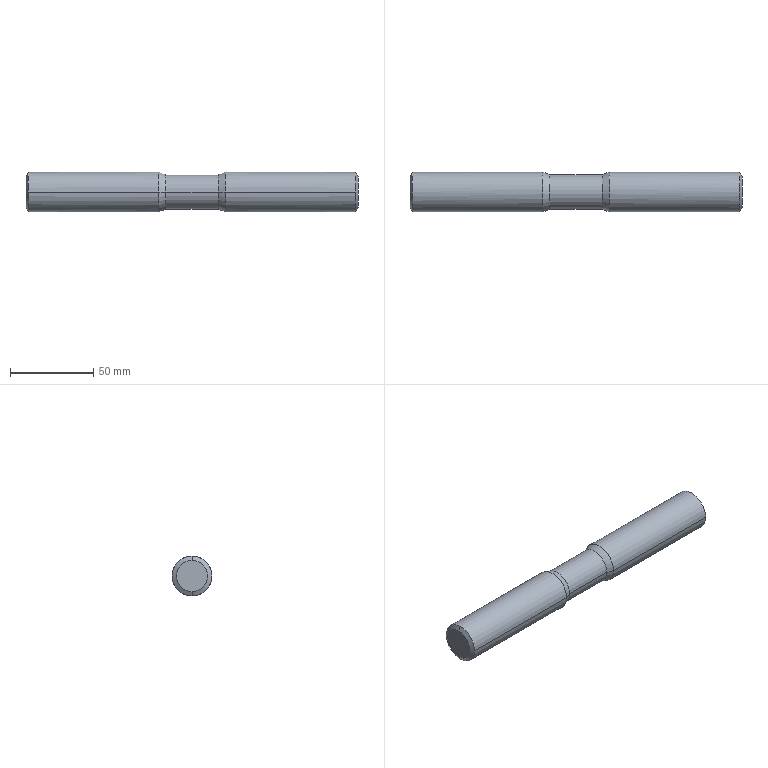Part | STEP file | GB/T901-1988 double-end stud, grade B, M24×200 | 1 solid | 16 faces | box 200 x 24 x 24 mm | volume 86144 mm3 | cone 8 | cylinder 6 | plane 2 | commonest cylinder face diameters 24 x4 20.784 x2
STEP:
#1=CARTESIAN_POINT('',(0.,0.,0.));
#2=DIRECTION('',(0.,0.,1.));
#3=DIRECTION('',(1.,0.,0.));
#4=AXIS2_PLACEMENT_3D('',#1,#2,#3);
#5=CARTESIAN_POINT('',(100.,0.,-9.402));
#6=VERTEX_POINT('',#5);
#7=CARTESIAN_POINT('',(100.,0.,9.402));
#8=VERTEX_POINT('',#7);
#9=CARTESIAN_POINT('',(100.,0.,0.));
#10=DIRECTION('',(-1.,0.,0.));
#11=DIRECTION('',(0.,0.,1.));
#12=AXIS2_PLACEMENT_3D('',#9,#10,#11);
#13=CIRCLE('',#12,9.402);
#14=CARTESIAN_POINT('',(100.,0.,0.));
#15=DIRECTION('',(-1.,0.,0.));
#16=DIRECTION('',(0.,0.,-1.));
#17=AXIS2_PLACEMENT_3D('',#14,#15,#16);
#18=CONICAL_SURFACE('',#17,9.402,1.047);
#19=CARTESIAN_POINT('',(-3.142,0.));
#20=DIRECTION('',(1.,0.));
#21=VECTOR('',#20,1.);
#22=LINE('',#19,#21);
#23=(GEOMETRIC_REPRESENTATION_CONTEXT(2)PARAMETRIC_REPRESENTATION_CONTEXT()REPRESENTATION_CONTEXT('',''));
#24=DEFINITIONAL_REPRESENTATION('',(#22),#23);
#25=PCURVE('',#18,#24);
#26=CARTESIAN_POINT('',(100.,12.,0.));
#27=DIRECTION('',(-1.,0.,0.));
#28=DIRECTION('',(0.,1.,0.));
#29=AXIS2_PLACEMENT_3D('',#26,#27,#28);
#30=PLANE('',#29);
#31=CARTESIAN_POINT('',(-12.,0.));
#32=DIRECTION('',(0.,-1.));
#33=AXIS2_PLACEMENT_2D('',#31,#32);
#34=CIRCLE('',#33,9.402);
#35=(GEOMETRIC_REPRESENTATION_CONTEXT(2)PARAMETRIC_REPRESENTATION_CONTEXT()REPRESENTATION_CONTEXT('',''));
#36=DEFINITIONAL_REPRESENTATION('',(#34),#35);
#37=PCURVE('',#30,#36);
#38=SURFACE_CURVE('',#13,(#25,#37),.PCURVE_S1.);
#39=EDGE_CURVE('',#6,#8,#38,.T.);
#40=ORIENTED_EDGE('',*,*,#39,.T.);
#41=CARTESIAN_POINT('',(98.5,0.,12.));
#42=VERTEX_POINT('',#41);
#43=CARTESIAN_POINT('',(100.,0.,9.402));
#44=DIRECTION('',(-0.5,0.,0.866));
#45=VECTOR('',#44,1.);
#46=LINE('',#43,#45);
#47=CARTESIAN_POINT('',(3.142,0.));
#48=DIRECTION('',(0.,1.));
#49=VECTOR('',#48,1.);
#50=LINE('',#47,#49);
#51=(GEOMETRIC_REPRESENTATION_CONTEXT(2)PARAMETRIC_REPRESENTATION_CONTEXT()REPRESENTATION_CONTEXT('',''));
#52=DEFINITIONAL_REPRESENTATION('',(#50),#51);
#53=PCURVE('',#18,#52);
#54=CARTESIAN_POINT('',(100.,0.,0.));
#55=DIRECTION('',(-1.,0.,0.));
#56=DIRECTION('',(0.,0.,-1.));
#57=AXIS2_PLACEMENT_3D('',#54,#55,#56);
#58=CONICAL_SURFACE('',#57,9.402,1.047);
#59=CARTESIAN_POINT('',(3.142,0.));
#60=DIRECTION('',(0.,1.));
#61=VECTOR('',#60,1.);
#62=LINE('',#59,#61);
#63=(GEOMETRIC_REPRESENTATION_CONTEXT(2)PARAMETRIC_REPRESENTATION_CONTEXT()REPRESENTATION_CONTEXT('',''));
#64=DEFINITIONAL_REPRESENTATION('',(#62),#63);
#65=PCURVE('',#58,#64);
#66=SURFACE_CURVE('',#46,(#53,#65),.PCURVE_S1.);
#67=EDGE_CURVE('',#8,#42,#66,.T.);
#68=ORIENTED_EDGE('',*,*,#67,.T.);
#69=CARTESIAN_POINT('',(98.5,-12.,0.));
#70=VERTEX_POINT('',#69);
#71=CARTESIAN_POINT('',(98.5,0.,0.));
#72=DIRECTION('',(-1.,0.,0.));
#73=DIRECTION('',(0.,0.,1.));
#74=AXIS2_PLACEMENT_3D('',#71,#72,#73);
#75=CIRCLE('',#74,12.);
#76=CARTESIAN_POINT('',(-3.142,1.5));
#77=DIRECTION('',(1.,0.));
#78=VECTOR('',#77,1.);
#79=LINE('',#76,#78);
#80=(GEOMETRIC_REPRESENTATION_CONTEXT(2)PARAMETRIC_REPRESENTATION_CONTEXT()REPRESENTATION_CONTEXT('',''));
#81=DEFINITIONAL_REPRESENTATION('',(#79),#80);
#82=PCURVE('',#18,#81);
#83=CARTESIAN_POINT('',(100.,0.,0.));
#84=DIRECTION('',(1.,0.,0.));
#85=DIRECTION('',(0.,-1.,0.));
#86=AXIS2_PLACEMENT_3D('',#83,#84,#85);
#87=CYLINDRICAL_SURFACE('',#86,12.);
#88=CARTESIAN_POINT('',(10.996,-1.5));
#89=DIRECTION('',(-1.,0.));
#90=VECTOR('',#89,1.);
#91=LINE('',#88,#90);
#92=(GEOMETRIC_REPRESENTATION_CONTEXT(2)PARAMETRIC_REPRESENTATION_CONTEXT()REPRESENTATION_CONTEXT('',''));
#93=DEFINITIONAL_REPRESENTATION('',(#91),#92);
#94=PCURVE('',#87,#93);
#95=SURFACE_CURVE('',#75,(#82,#94),.PCURVE_S1.);
#96=EDGE_CURVE('',#70,#42,#95,.T.);
#97=ORIENTED_EDGE('',*,*,#96,.F.);
#98=CARTESIAN_POINT('',(98.5,0.,-12.));
#99=VERTEX_POINT('',#98);
#100=CARTESIAN_POINT('',(98.5,0.,0.));
#101=DIRECTION('',(-1.,0.,0.));
#102=DIRECTION('',(0.,0.,1.));
#103=AXIS2_PLACEMENT_3D('',#100,#101,#102);
#104=CIRCLE('',#103,12.);
#105=CARTESIAN_POINT('',(-3.142,1.5));
#106=DIRECTION('',(1.,0.));
#107=VECTOR('',#106,1.);
#108=LINE('',#105,#107);
#109=(GEOMETRIC_REPRESENTATION_CONTEXT(2)PARAMETRIC_REPRESENTATION_CONTEXT()REPRESENTATION_CONTEXT('',''));
#110=DEFINITIONAL_REPRESENTATION('',(#108),#109);
#111=PCURVE('',#18,#110);
#112=CARTESIAN_POINT('',(100.,0.,0.));
#113=DIRECTION('',(1.,0.,0.));
#114=DIRECTION('',(0.,-1.,0.));
#115=AXIS2_PLACEMENT_3D('',#112,#113,#114);
#116=CYLINDRICAL_SURFACE('',#115,12.);
#117=CARTESIAN_POINT('',(4.712,-1.5));
#118=DIRECTION('',(-1.,0.));
#119=VECTOR('',#118,1.);
#120=LINE('',#117,#119);
#121=(GEOMETRIC_REPRESENTATION_CONTEXT(2)PARAMETRIC_REPRESENTATION_CONTEXT()REPRESENTATION_CONTEXT('',''));
#122=DEFINITIONAL_REPRESENTATION('',(#120),#121);
#123=PCURVE('',#116,#122);
#124=SURFACE_CURVE('',#104,(#111,#123),.PCURVE_S1.);
#125=EDGE_CURVE('',#99,#70,#124,.T.);
#126=ORIENTED_EDGE('',*,*,#125,.F.);
#127=CARTESIAN_POINT('',(100.,0.,-9.402));
#128=DIRECTION('',(-0.5,0.,-0.866));
#129=VECTOR('',#128,1.);
#130=LINE('',#127,#129);
#131=CARTESIAN_POINT('',(0.,0.));
#132=DIRECTION('',(0.,1.));
#133=VECTOR('',#132,1.);
#134=LINE('',#131,#133);
#135=(GEOMETRIC_REPRESENTATION_CONTEXT(2)PARAMETRIC_REPRESENTATION_CONTEXT()REPRESENTATION_CONTEXT('',''));
#136=DEFINITIONAL_REPRESENTATION('',(#134),#135);
#137=PCURVE('',#18,#136);
#138=CARTESIAN_POINT('',(6.283,0.));
#139=DIRECTION('',(0.,1.));
#140=VECTOR('',#139,1.);
#141=LINE('',#138,#140);
#142=(GEOMETRIC_REPRESENTATION_CONTEXT(2)PARAMETRIC_REPRESENTATION_CONTEXT()REPRESENTATION_CONTEXT('',''));
#143=DEFINITIONAL_REPRESENTATION('',(#141),#142);
#144=PCURVE('',#58,#143);
#145=SURFACE_CURVE('',#130,(#137,#144),.PCURVE_S1.);
#146=EDGE_CURVE('',#6,#99,#145,.T.);
#147=ORIENTED_EDGE('',*,*,#146,.F.);
#148=EDGE_LOOP('',(#40,#68,#97,#126,#147));
#149=FACE_BOUND('',#148,.T.);
#150=ADVANCED_FACE('',(#149),#18,.T.);
#151=CARTESIAN_POINT('',(15.8,10.392,0.));
#152=VERTEX_POINT('',#151);
#153=CARTESIAN_POINT('',(15.8,-10.392,0.));
#154=VERTEX_POINT('',#153);
#155=CARTESIAN_POINT('',(15.8,0.,0.));
#156=DIRECTION('',(-1.,0.,0.));
#157=DIRECTION('',(0.,-1.,0.));
#158=AXIS2_PLACEMENT_3D('',#155,#156,#157);
#159=CIRCLE('',#158,10.392);
#160=CARTESIAN_POINT('',(15.8,0.,0.));
#161=DIRECTION('',(1.,0.,0.));
#162=DIRECTION('',(0.,-1.,0.));
#163=AXIS2_PLACEMENT_3D('',#160,#161,#162);
#164=CONICAL_SURFACE('',#163,10.392,0.3656);
#165=CARTESIAN_POINT('',(6.283,0.));
#166=DIRECTION('',(-1.,0.));
#167=VECTOR('',#166,1.);
#168=LINE('',#165,#167);
#169=(GEOMETRIC_REPRESENTATION_CONTEXT(2)PARAMETRIC_REPRESENTATION_CONTEXT()REPRESENTATION_CONTEXT('',''));
#170=DEFINITIONAL_REPRESENTATION('',(#168),#169);
#171=PCURVE('',#164,#170);
#172=CARTESIAN_POINT('',(-100.,0.,0.));
#173=DIRECTION('',(-1.,0.,0.));
#174=DIRECTION('',(0.,-1.,0.));
#175=AXIS2_PLACEMENT_3D('',#172,#173,#174);
#176=CYLINDRICAL_SURFACE('',#175,10.392);
#177=CARTESIAN_POINT('',(0.,-115.8));
#178=DIRECTION('',(1.,0.));
#179=VECTOR('',#178,1.);
#180=LINE('',#177,#179);
#181=(GEOMETRIC_REPRESENTATION_CONTEXT(2)PARAMETRIC_REPRESENTATION_CONTEXT()REPRESENTATION_CONTEXT('',''));
#182=DEFINITIONAL_REPRESENTATION('',(#180),#181);
#183=PCURVE('',#176,#182);
#184=SURFACE_CURVE('',#159,(#171,#183),.PCURVE_S1.);
#185=EDGE_CURVE('',#152,#154,#184,.T.);
#186=ORIENTED_EDGE('',*,*,#185,.F.);
#187=CARTESIAN_POINT('',(20.,12.,0.));
#188=VERTEX_POINT('',#187);
#189=CARTESIAN_POINT('',(15.8,10.392,0.));
#190=DIRECTION('',(0.9339,0.3575,0.));
#191=VECTOR('',#190,1.);
#192=LINE('',#189,#191);
#193=CARTESIAN_POINT('',(3.142,0.));
#194=DIRECTION('',(0.,1.));
#195=VECTOR('',#194,1.);
#196=LINE('',#193,#195);
#197=(GEOMETRIC_REPRESENTATION_CONTEXT(2)PARAMETRIC_REPRESENTATION_CONTEXT()REPRESENTATION_CONTEXT('',''));
#198=DEFINITIONAL_REPRESENTATION('',(#196),#197);
#199=PCURVE('',#164,#198);
#200=CARTESIAN_POINT('',(15.8,0.,0.));
#201=DIRECTION('',(1.,0.,0.));
#202=DIRECTION('',(0.,-1.,0.));
#203=AXIS2_PLACEMENT_3D('',#200,#201,#202);
#204=CONICAL_SURFACE('',#203,10.392,0.3656);
#205=CARTESIAN_POINT('',(3.142,0.));
#206=DIRECTION('',(0.,1.));
#207=VECTOR('',#206,1.);
#208=LINE('',#205,#207);
#209=(GEOMETRIC_REPRESENTATION_CONTEXT(2)PARAMETRIC_REPRESENTATION_CONTEXT()REPRESENTATION_CONTEXT('',''));
#210=DEFINITIONAL_REPRESENTATION('',(#208),#209);
#211=PCURVE('',#204,#210);
#212=SURFACE_CURVE('',#192,(#199,#211),.PCURVE_S1.);
#213=EDGE_CURVE('',#152,#188,#212,.T.);
#214=ORIENTED_EDGE('',*,*,#213,.T.);
#215=CARTESIAN_POINT('',(20.,-12.,0.));
#216=VERTEX_POINT('',#215);
#217=CARTESIAN_POINT('',(20.,0.,0.));
#218=DIRECTION('',(-1.,0.,0.));
#219=DIRECTION('',(0.,-1.,0.));
#220=AXIS2_PLACEMENT_3D('',#217,#218,#219);
#221=CIRCLE('',#220,12.);
#222=CARTESIAN_POINT('',(6.283,4.2));
#223=DIRECTION('',(-1.,0.));
#224=VECTOR('',#223,1.);
#225=LINE('',#222,#224);
#226=(GEOMETRIC_REPRESENTATION_CONTEXT(2)PARAMETRIC_REPRESENTATION_CONTEXT()REPRESENTATION_CONTEXT('',''));
#227=DEFINITIONAL_REPRESENTATION('',(#225),#226);
#228=PCURVE('',#164,#227);
#229=CARTESIAN_POINT('',(6.283,-80.));
#230=DIRECTION('',(-1.,0.));
#231=VECTOR('',#230,1.);
#232=LINE('',#229,#231);
#233=(GEOMETRIC_REPRESENTATION_CONTEXT(2)PARAMETRIC_REPRESENTATION_CONTEXT()REPRESENTATION_CONTEXT('',''));
#234=DEFINITIONAL_REPRESENTATION('',(#232),#233);
#235=PCURVE('',#116,#234);
#236=SURFACE_CURVE('',#221,(#228,#235),.PCURVE_S1.);
#237=EDGE_CURVE('',#188,#216,#236,.T.);
#238=ORIENTED_EDGE('',*,*,#237,.T.);
#239=CARTESIAN_POINT('',(15.8,-10.392,0.));
#240=DIRECTION('',(0.9339,-0.3575,0.));
#241=VECTOR('',#240,1.);
#242=LINE('',#239,#241);
#243=CARTESIAN_POINT('',(0.,0.));
#244=DIRECTION('',(0.,1.));
#245=VECTOR('',#244,1.);
#246=LINE('',#243,#245);
#247=(GEOMETRIC_REPRESENTATION_CONTEXT(2)PARAMETRIC_REPRESENTATION_CONTEXT()REPRESENTATION_CONTEXT('',''));
#248=DEFINITIONAL_REPRESENTATION('',(#246),#247);
#249=PCURVE('',#164,#248);
#250=CARTESIAN_POINT('',(6.283,0.));
#251=DIRECTION('',(0.,1.));
#252=VECTOR('',#251,1.);
#253=LINE('',#250,#252);
#254=(GEOMETRIC_REPRESENTATION_CONTEXT(2)PARAMETRIC_REPRESENTATION_CONTEXT()REPRESENTATION_CONTEXT('',''));
#255=DEFINITIONAL_REPRESENTATION('',(#253),#254);
#256=PCURVE('',#204,#255);
#257=SURFACE_CURVE('',#242,(#249,#256),.PCURVE_S1.);
#258=EDGE_CURVE('',#154,#216,#257,.T.);
#259=ORIENTED_EDGE('',*,*,#258,.F.);
#260=EDGE_LOOP('',(#186,#214,#238,#259));
#261=FACE_BOUND('',#260,.T.);
#262=ADVANCED_FACE('',(#261),#164,.T.);
#263=ORIENTED_EDGE('',*,*,#237,.F.);
#264=CARTESIAN_POINT('',(98.5,12.,0.));
#265=VERTEX_POINT('',#264);
#266=CARTESIAN_POINT('',(100.,12.,0.));
#267=DIRECTION('',(1.,0.,0.));
#268=VECTOR('',#267,1.);
#269=LINE('',#266,#268);
#270=CARTESIAN_POINT('',(3.142,0.));
#271=DIRECTION('',(0.,1.));
#272=VECTOR('',#271,1.);
#273=LINE('',#270,#272);
#274=(GEOMETRIC_REPRESENTATION_CONTEXT(2)PARAMETRIC_REPRESENTATION_CONTEXT()REPRESENTATION_CONTEXT('',''));
#275=DEFINITIONAL_REPRESENTATION('',(#273),#274);
#276=PCURVE('',#116,#275);
#277=CARTESIAN_POINT('',(3.142,0.));
#278=DIRECTION('',(0.,1.));
#279=VECTOR('',#278,1.);
#280=LINE('',#277,#279);
#281=(GEOMETRIC_REPRESENTATION_CONTEXT(2)PARAMETRIC_REPRESENTATION_CONTEXT()REPRESENTATION_CONTEXT('',''));
#282=DEFINITIONAL_REPRESENTATION('',(#280),#281);
#283=PCURVE('',#87,#282);
#284=SURFACE_CURVE('',#269,(#276,#283),.PCURVE_S1.);
#285=EDGE_CURVE('',#188,#265,#284,.T.);
#286=ORIENTED_EDGE('',*,*,#285,.T.);
#287=CARTESIAN_POINT('',(98.5,0.,0.));
#288=DIRECTION('',(-1.,0.,0.));
#289=DIRECTION('',(0.,0.,1.));
#290=AXIS2_PLACEMENT_3D('',#287,#288,#289);
#291=CIRCLE('',#290,12.);
#292=CARTESIAN_POINT('',(4.712,-1.5));
#293=DIRECTION('',(-1.,0.));
#294=VECTOR('',#293,1.);
#295=LINE('',#292,#294);
#296=(GEOMETRIC_REPRESENTATION_CONTEXT(2)PARAMETRIC_REPRESENTATION_CONTEXT()REPRESENTATION_CONTEXT('',''));
#297=DEFINITIONAL_REPRESENTATION('',(#295),#296);
#298=PCURVE('',#116,#297);
#299=CARTESIAN_POINT('',(3.142,1.5));
#300=DIRECTION('',(1.,0.));
#301=VECTOR('',#300,1.);
#302=LINE('',#299,#301);
#303=(GEOMETRIC_REPRESENTATION_CONTEXT(2)PARAMETRIC_REPRESENTATION_CONTEXT()REPRESENTATION_CONTEXT('',''));
#304=DEFINITIONAL_REPRESENTATION('',(#302),#303);
#305=PCURVE('',#58,#304);
#306=SURFACE_CURVE('',#291,(#298,#305),.PCURVE_S1.);
#307=EDGE_CURVE('',#265,#99,#306,.T.);
#308=ORIENTED_EDGE('',*,*,#307,.T.);
#309=ORIENTED_EDGE('',*,*,#125,.T.);
#310=CARTESIAN_POINT('',(100.,-12.,0.));
#311=DIRECTION('',(1.,0.,0.));
#312=VECTOR('',#311,1.);
#313=LINE('',#310,#312);
#314=CARTESIAN_POINT('',(0.,0.));
#315=DIRECTION('',(0.,1.));
#316=VECTOR('',#315,1.);
#317=LINE('',#314,#316);
#318=(GEOMETRIC_REPRESENTATION_CONTEXT(2)PARAMETRIC_REPRESENTATION_CONTEXT()REPRESENTATION_CONTEXT('',''));
#319=DEFINITIONAL_REPRESENTATION('',(#317),#318);
#320=PCURVE('',#116,#319);
#321=CARTESIAN_POINT('',(6.283,0.));
#322=DIRECTION('',(0.,1.));
#323=VECTOR('',#322,1.);
#324=LINE('',#321,#323);
#325=(GEOMETRIC_REPRESENTATION_CONTEXT(2)PARAMETRIC_REPRESENTATION_CONTEXT()REPRESENTATION_CONTEXT('',''));
#326=DEFINITIONAL_REPRESENTATION('',(#324),#325);
#327=PCURVE('',#87,#326);
#328=SURFACE_CURVE('',#313,(#320,#327),.PCURVE_S1.);
#329=EDGE_CURVE('',#216,#70,#328,.T.);
#330=ORIENTED_EDGE('',*,*,#329,.F.);
#331=EDGE_LOOP('',(#263,#286,#308,#309,#330));
#332=FACE_BOUND('',#331,.T.);
#333=ADVANCED_FACE('',(#332),#116,.T.);
#334=CARTESIAN_POINT('',(-100.,0.,9.402));
#335=VERTEX_POINT('',#334);
#336=CARTESIAN_POINT('',(-100.,0.,-9.402));
#337=VERTEX_POINT('',#336);
#338=CARTESIAN_POINT('',(-100.,0.,0.));
#339=DIRECTION('',(-1.,0.,0.));
#340=DIRECTION('',(0.,0.,1.));
#341=AXIS2_PLACEMENT_3D('',#338,#339,#340);
#342=CIRCLE('',#341,9.402);
#343=CARTESIAN_POINT('',(-100.,0.,0.));
#344=DIRECTION('',(1.,0.,0.));
#345=DIRECTION('',(0.,0.,-1.));
#346=AXIS2_PLACEMENT_3D('',#343,#344,#345);
#347=CONICAL_SURFACE('',#346,9.402,1.047);
#348=CARTESIAN_POINT('',(3.142,0.));
#349=DIRECTION('',(-1.,0.));
#350=VECTOR('',#349,1.);
#351=LINE('',#348,#350);
#352=(GEOMETRIC_REPRESENTATION_CONTEXT(2)PARAMETRIC_REPRESENTATION_CONTEXT()REPRESENTATION_CONTEXT('',''));
#353=DEFINITIONAL_REPRESENTATION('',(#351),#352);
#354=PCURVE('',#347,#353);
#355=CARTESIAN_POINT('',(-100.,12.,0.));
#356=DIRECTION('',(1.,0.,0.));
#357=DIRECTION('',(0.,1.,0.));
#358=AXIS2_PLACEMENT_3D('',#355,#356,#357);
#359=PLANE('',#358);
#360=CARTESIAN_POINT('',(-12.,9.402));
#361=CARTESIAN_POINT('',(4.285,9.402));
#362=CARTESIAN_POINT('',(-3.858,-4.701));
#363=CARTESIAN_POINT('',(-12.,-18.804));
#364=CARTESIAN_POINT('',(-20.142,-4.701));
#365=CARTESIAN_POINT('',(-28.285,9.402));
#366=CARTESIAN_POINT('',(-12.,9.402));
#367=(BOUNDED_CURVE()B_SPLINE_CURVE(2,(#360,#361,#362,#363,#364,#365,#366),.UNSPECIFIED.,.T.,.F.)B_SPLINE_CURVE_WITH_KNOTS((1,2,2,2,2,1),(-2.094,0.,2.094,4.189,6.283,8.378),.UNSPECIFIED.)CURVE()GEOMETRIC_REPRESENTATION_ITEM()RATIONAL_B_SPLINE_CURVE((1.,0.5,1.,0.5,1.,0.5,1.))REPRESENTATION_ITEM(''));
#368=(GEOMETRIC_REPRESENTATION_CONTEXT(2)PARAMETRIC_REPRESENTATION_CONTEXT()REPRESENTATION_CONTEXT('',''));
#369=DEFINITIONAL_REPRESENTATION('',(#367),#368);
#370=PCURVE('',#359,#369);
#371=SURFACE_CURVE('',#342,(#354,#370),.PCURVE_S1.);
#372=EDGE_CURVE('',#335,#337,#371,.T.);
#373=ORIENTED_EDGE('',*,*,#372,.F.);
#374=CARTESIAN_POINT('',(-98.5,0.,12.));
#375=VERTEX_POINT('',#374);
#376=CARTESIAN_POINT('',(-100.,0.,9.402));
#377=DIRECTION('',(0.5,0.,0.866));
#378=VECTOR('',#377,1.);
#379=LINE('',#376,#378);
#380=CARTESIAN_POINT('',(3.142,0.));
#381=DIRECTION('',(0.,1.));
#382=VECTOR('',#381,1.);
#383=LINE('',#380,#382);
#384=(GEOMETRIC_REPRESENTATION_CONTEXT(2)PARAMETRIC_REPRESENTATION_CONTEXT()REPRESENTATION_CONTEXT('',''));
#385=DEFINITIONAL_REPRESENTATION('',(#383),#384);
#386=PCURVE('',#347,#385);
#387=CARTESIAN_POINT('',(-100.,0.,0.));
#388=DIRECTION('',(1.,0.,0.));
#389=DIRECTION('',(0.,0.,-1.));
#390=AXIS2_PLACEMENT_3D('',#387,#388,#389);
#391=CONICAL_SURFACE('',#390,9.402,1.047);
#392=CARTESIAN_POINT('',(3.142,0.));
#393=DIRECTION('',(0.,1.));
#394=VECTOR('',#393,1.);
#395=LINE('',#392,#394);
#396=(GEOMETRIC_REPRESENTATION_CONTEXT(2)PARAMETRIC_REPRESENTATION_CONTEXT()REPRESENTATION_CONTEXT('',''));
#397=DEFINITIONAL_REPRESENTATION('',(#395),#396);
#398=PCURVE('',#391,#397);
#399=SURFACE_CURVE('',#379,(#386,#398),.PCURVE_S1.);
#400=EDGE_CURVE('',#335,#375,#399,.T.);
#401=ORIENTED_EDGE('',*,*,#400,.T.);
#402=CARTESIAN_POINT('',(-98.5,12.,0.));
#403=VERTEX_POINT('',#402);
#404=CARTESIAN_POINT('',(-98.5,0.,0.));
#405=DIRECTION('',(-1.,0.,0.));
#406=DIRECTION('',(0.,0.,1.));
#407=AXIS2_PLACEMENT_3D('',#404,#405,#406);
#408=CIRCLE('',#407,12.);
#409=CARTESIAN_POINT('',(3.142,1.5));
#410=DIRECTION('',(-1.,0.));
#411=VECTOR('',#410,1.);
#412=LINE('',#409,#411);
#413=(GEOMETRIC_REPRESENTATION_CONTEXT(2)PARAMETRIC_REPRESENTATION_CONTEXT()REPRESENTATION_CONTEXT('',''));
#414=DEFINITIONAL_REPRESENTATION('',(#412),#413);
#415=PCURVE('',#347,#414);
#416=CARTESIAN_POINT('',(-100.,0.,0.));
#417=DIRECTION('',(-1.,0.,0.));
#418=DIRECTION('',(0.,-1.,0.));
#419=AXIS2_PLACEMENT_3D('',#416,#417,#418);
#420=CYLINDRICAL_SURFACE('',#419,12.);
#421=CARTESIAN_POINT('',(1.571,-1.5));
#422=DIRECTION('',(1.,0.));
#423=VECTOR('',#422,1.);
#424=LINE('',#421,#423);
#425=(GEOMETRIC_REPRESENTATION_CONTEXT(2)PARAMETRIC_REPRESENTATION_CONTEXT()REPRESENTATION_CONTEXT('',''));
#426=DEFINITIONAL_REPRESENTATION('',(#424),#425);
#427=PCURVE('',#420,#426);
#428=SURFACE_CURVE('',#408,(#415,#427),.PCURVE_S1.);
#429=EDGE_CURVE('',#375,#403,#428,.T.);
#430=ORIENTED_EDGE('',*,*,#429,.T.);
#431=CARTESIAN_POINT('',(-98.5,0.,-12.));
#432=VERTEX_POINT('',#431);
#433=CARTESIAN_POINT('',(-98.5,0.,0.));
#434=DIRECTION('',(-1.,0.,0.));
#435=DIRECTION('',(0.,0.,1.));
#436=AXIS2_PLACEMENT_3D('',#433,#434,#435);
#437=CIRCLE('',#436,12.);
#438=CARTESIAN_POINT('',(3.142,1.5));
#439=DIRECTION('',(-1.,0.));
#440=VECTOR('',#439,1.);
#441=LINE('',#438,#440);
#442=(GEOMETRIC_REPRESENTATION_CONTEXT(2)PARAMETRIC_REPRESENTATION_CONTEXT()REPRESENTATION_CONTEXT('',''));
#443=DEFINITIONAL_REPRESENTATION('',(#441),#442);
#444=PCURVE('',#347,#443);
#445=CARTESIAN_POINT('',(-100.,0.,0.));
#446=DIRECTION('',(-1.,0.,0.));
#447=DIRECTION('',(0.,-1.,0.));
#448=AXIS2_PLACEMENT_3D('',#445,#446,#447);
#449=CYLINDRICAL_SURFACE('',#448,12.);
#450=CARTESIAN_POINT('',(1.571,-1.5));
#451=DIRECTION('',(1.,0.));
#452=VECTOR('',#451,1.);
#453=LINE('',#450,#452);
#454=(GEOMETRIC_REPRESENTATION_CONTEXT(2)PARAMETRIC_REPRESENTATION_CONTEXT()REPRESENTATION_CONTEXT('',''));
#455=DEFINITIONAL_REPRESENTATION('',(#453),#454);
#456=PCURVE('',#449,#455);
#457=SURFACE_CURVE('',#437,(#444,#456),.PCURVE_S1.);
#458=EDGE_CURVE('',#403,#432,#457,.T.);
#459=ORIENTED_EDGE('',*,*,#458,.T.);
#460=CARTESIAN_POINT('',(-100.,0.,-9.402));
#461=DIRECTION('',(0.5,0.,-0.866));
#462=VECTOR('',#461,1.);
#463=LINE('',#460,#462);
#464=CARTESIAN_POINT('',(0.,0.));
#465=DIRECTION('',(0.,1.));
#466=VECTOR('',#465,1.);
#467=LINE('',#464,#466);
#468=(GEOMETRIC_REPRESENTATION_CONTEXT(2)PARAMETRIC_REPRESENTATION_CONTEXT()REPRESENTATION_CONTEXT('',''));
#469=DEFINITIONAL_REPRESENTATION('',(#467),#468);
#470=PCURVE('',#347,#469);
#471=CARTESIAN_POINT('',(6.283,0.));
#472=DIRECTION('',(0.,1.));
#473=VECTOR('',#472,1.);
#474=LINE('',#471,#473);
#475=(GEOMETRIC_REPRESENTATION_CONTEXT(2)PARAMETRIC_REPRESENTATION_CONTEXT()REPRESENTATION_CONTEXT('',''));
#476=DEFINITIONAL_REPRESENTATION('',(#474),#475);
#477=PCURVE('',#391,#476);
#478=SURFACE_CURVE('',#463,(#470,#477),.PCURVE_S1.);
#479=EDGE_CURVE('',#337,#432,#478,.T.);
#480=ORIENTED_EDGE('',*,*,#479,.F.);
#481=EDGE_LOOP('',(#373,#401,#430,#459,#480));
#482=FACE_BOUND('',#481,.T.);
#483=ADVANCED_FACE('',(#482),#347,.T.);
#484=CARTESIAN_POINT('',(-15.8,-10.392,0.));
#485=VERTEX_POINT('',#484);
#486=CARTESIAN_POINT('',(-15.8,10.392,0.));
#487=VERTEX_POINT('',#486);
#488=CARTESIAN_POINT('',(-15.8,0.,0.));
#489=DIRECTION('',(-1.,0.,0.));
#490=DIRECTION('',(0.,-1.,0.));
#491=AXIS2_PLACEMENT_3D('',#488,#489,#490);
#492=CIRCLE('',#491,10.392);
#493=CARTESIAN_POINT('',(-15.8,0.,0.));
#494=DIRECTION('',(-1.,0.,0.));
#495=DIRECTION('',(0.,-1.,0.));
#496=AXIS2_PLACEMENT_3D('',#493,#494,#495);
#497=CONICAL_SURFACE('',#496,10.392,0.3656);
#498=CARTESIAN_POINT('',(0.,0.));
#499=DIRECTION('',(1.,0.));
#500=VECTOR('',#499,1.);
#501=LINE('',#498,#500);
#502=(GEOMETRIC_REPRESENTATION_CONTEXT(2)PARAMETRIC_REPRESENTATION_CONTEXT()REPRESENTATION_CONTEXT('',''));
#503=DEFINITIONAL_REPRESENTATION('',(#501),#502);
#504=PCURVE('',#497,#503);
#505=CARTESIAN_POINT('',(-100.,0.,0.));
#506=DIRECTION('',(-1.,0.,0.));
#507=DIRECTION('',(0.,-1.,0.));
#508=AXIS2_PLACEMENT_3D('',#505,#506,#507);
#509=CYLINDRICAL_SURFACE('',#508,10.392);
#510=CARTESIAN_POINT('',(0.,-84.2));
#511=DIRECTION('',(1.,0.));
#512=VECTOR('',#511,1.);
#513=LINE('',#510,#512);
#514=(GEOMETRIC_REPRESENTATION_CONTEXT(2)PARAMETRIC_REPRESENTATION_CONTEXT()REPRESENTATION_CONTEXT('',''));
#515=DEFINITIONAL_REPRESENTATION('',(#513),#514);
#516=PCURVE('',#509,#515);
#517=SURFACE_CURVE('',#492,(#504,#516),.PCURVE_S1.);
#518=EDGE_CURVE('',#485,#487,#517,.T.);
#519=ORIENTED_EDGE('',*,*,#518,.T.);
#520=CARTESIAN_POINT('',(-20.,12.,0.));
#521=VERTEX_POINT('',#520);
#522=CARTESIAN_POINT('',(-15.8,10.392,0.));
#523=DIRECTION('',(-0.9339,0.3575,0.));
#524=VECTOR('',#523,1.);
#525=LINE('',#522,#524);
#526=CARTESIAN_POINT('',(3.142,0.));
#527=DIRECTION('',(0.,1.));
#528=VECTOR('',#527,1.);
#529=LINE('',#526,#528);
#530=(GEOMETRIC_REPRESENTATION_CONTEXT(2)PARAMETRIC_REPRESENTATION_CONTEXT()REPRESENTATION_CONTEXT('',''));
#531=DEFINITIONAL_REPRESENTATION('',(#529),#530);
#532=PCURVE('',#497,#531);
#533=CARTESIAN_POINT('',(-15.8,0.,0.));
#534=DIRECTION('',(-1.,0.,0.));
#535=DIRECTION('',(0.,-1.,0.));
#536=AXIS2_PLACEMENT_3D('',#533,#534,#535);
#537=CONICAL_SURFACE('',#536,10.392,0.3656);
#538=CARTESIAN_POINT('',(3.142,0.));
#539=DIRECTION('',(0.,1.));
#540=VECTOR('',#539,1.);
#541=LINE('',#538,#540);
#542=(GEOMETRIC_REPRESENTATION_CONTEXT(2)PARAMETRIC_REPRESENTATION_CONTEXT()REPRESENTATION_CONTEXT('',''));
#543=DEFINITIONAL_REPRESENTATION('',(#541),#542);
#544=PCURVE('',#537,#543);
#545=SURFACE_CURVE('',#525,(#532,#544),.PCURVE_S1.);
#546=EDGE_CURVE('',#487,#521,#545,.T.);
#547=ORIENTED_EDGE('',*,*,#546,.T.);
#548=CARTESIAN_POINT('',(-20.,-12.,0.));
#549=VERTEX_POINT('',#548);
#550=CARTESIAN_POINT('',(-20.,0.,0.));
#551=DIRECTION('',(-1.,0.,0.));
#552=DIRECTION('',(0.,-1.,0.));
#553=AXIS2_PLACEMENT_3D('',#550,#551,#552);
#554=CIRCLE('',#553,12.);
#555=CARTESIAN_POINT('',(0.,4.2));
#556=DIRECTION('',(1.,0.));
#557=VECTOR('',#556,1.);
#558=LINE('',#555,#557);
#559=(GEOMETRIC_REPRESENTATION_CONTEXT(2)PARAMETRIC_REPRESENTATION_CONTEXT()REPRESENTATION_CONTEXT('',''));
#560=DEFINITIONAL_REPRESENTATION('',(#558),#559);
#561=PCURVE('',#497,#560);
#562=CARTESIAN_POINT('',(0.,-80.));
#563=DIRECTION('',(1.,0.));
#564=VECTOR('',#563,1.);
#565=LINE('',#562,#564);
#566=(GEOMETRIC_REPRESENTATION_CONTEXT(2)PARAMETRIC_REPRESENTATION_CONTEXT()REPRESENTATION_CONTEXT('',''));
#567=DEFINITIONAL_REPRESENTATION('',(#565),#566);
#568=PCURVE('',#420,#567);
#569=SURFACE_CURVE('',#554,(#561,#568),.PCURVE_S1.);
#570=EDGE_CURVE('',#549,#521,#569,.T.);
#571=ORIENTED_EDGE('',*,*,#570,.F.);
#572=CARTESIAN_POINT('',(-15.8,-10.392,0.));
#573=DIRECTION('',(-0.9339,-0.3575,0.));
#574=VECTOR('',#573,1.);
#575=LINE('',#572,#574);
#576=CARTESIAN_POINT('',(0.,0.));
#577=DIRECTION('',(0.,1.));
#578=VECTOR('',#577,1.);
#579=LINE('',#576,#578);
#580=(GEOMETRIC_REPRESENTATION_CONTEXT(2)PARAMETRIC_REPRESENTATION_CONTEXT()REPRESENTATION_CONTEXT('',''));
#581=DEFINITIONAL_REPRESENTATION('',(#579),#580);
#582=PCURVE('',#497,#581);
#583=CARTESIAN_POINT('',(6.283,0.));
#584=DIRECTION('',(0.,1.));
#585=VECTOR('',#584,1.);
#586=LINE('',#583,#585);
#587=(GEOMETRIC_REPRESENTATION_CONTEXT(2)PARAMETRIC_REPRESENTATION_CONTEXT()REPRESENTATION_CONTEXT('',''));
#588=DEFINITIONAL_REPRESENTATION('',(#586),#587);
#589=PCURVE('',#537,#588);
#590=SURFACE_CURVE('',#575,(#582,#589),.PCURVE_S1.);
#591=EDGE_CURVE('',#485,#549,#590,.T.);
#592=ORIENTED_EDGE('',*,*,#591,.F.);
#593=EDGE_LOOP('',(#519,#547,#571,#592));
#594=FACE_BOUND('',#593,.T.);
#595=ADVANCED_FACE('',(#594),#497,.T.);
#596=CARTESIAN_POINT('',(15.8,0.,0.));
#597=DIRECTION('',(-1.,0.,0.));
#598=DIRECTION('',(0.,-1.,0.));
#599=AXIS2_PLACEMENT_3D('',#596,#597,#598);
#600=CIRCLE('',#599,10.392);
#601=CARTESIAN_POINT('',(0.,-115.8));
#602=DIRECTION('',(1.,0.));
#603=VECTOR('',#602,1.);
#604=LINE('',#601,#603);
#605=(GEOMETRIC_REPRESENTATION_CONTEXT(2)PARAMETRIC_REPRESENTATION_CONTEXT()REPRESENTATION_CONTEXT('',''));
#606=DEFINITIONAL_REPRESENTATION('',(#604),#605);
#607=PCURVE('',#509,#606);
#608=CARTESIAN_POINT('',(6.283,0.));
#609=DIRECTION('',(-1.,0.));
#610=VECTOR('',#609,1.);
#611=LINE('',#608,#610);
#612=(GEOMETRIC_REPRESENTATION_CONTEXT(2)PARAMETRIC_REPRESENTATION_CONTEXT()REPRESENTATION_CONTEXT('',''));
#613=DEFINITIONAL_REPRESENTATION('',(#611),#612);
#614=PCURVE('',#204,#613);
#615=SURFACE_CURVE('',#600,(#607,#614),.PCURVE_S1.);
#616=EDGE_CURVE('',#154,#152,#615,.T.);
#617=ORIENTED_EDGE('',*,*,#616,.T.);
#618=CARTESIAN_POINT('',(-100.,10.392,0.));
#619=DIRECTION('',(-1.,0.,0.));
#620=VECTOR('',#619,1.);
#621=LINE('',#618,#620);
#622=CARTESIAN_POINT('',(3.142,0.));
#623=DIRECTION('',(0.,1.));
#624=VECTOR('',#623,1.);
#625=LINE('',#622,#624);
#626=(GEOMETRIC_REPRESENTATION_CONTEXT(2)PARAMETRIC_REPRESENTATION_CONTEXT()REPRESENTATION_CONTEXT('',''));
#627=DEFINITIONAL_REPRESENTATION('',(#625),#626);
#628=PCURVE('',#509,#627);
#629=CARTESIAN_POINT('',(3.142,0.));
#630=DIRECTION('',(0.,1.));
#631=VECTOR('',#630,1.);
#632=LINE('',#629,#631);
#633=(GEOMETRIC_REPRESENTATION_CONTEXT(2)PARAMETRIC_REPRESENTATION_CONTEXT()REPRESENTATION_CONTEXT('',''));
#634=DEFINITIONAL_REPRESENTATION('',(#632),#633);
#635=PCURVE('',#176,#634);
#636=SURFACE_CURVE('',#621,(#628,#635),.PCURVE_S1.);
#637=EDGE_CURVE('',#152,#487,#636,.T.);
#638=ORIENTED_EDGE('',*,*,#637,.T.);
#639=ORIENTED_EDGE('',*,*,#518,.F.);
#640=CARTESIAN_POINT('',(-100.,-10.392,0.));
#641=DIRECTION('',(-1.,0.,0.));
#642=VECTOR('',#641,1.);
#643=LINE('',#640,#642);
#644=CARTESIAN_POINT('',(0.,0.));
#645=DIRECTION('',(0.,1.));
#646=VECTOR('',#645,1.);
#647=LINE('',#644,#646);
#648=(GEOMETRIC_REPRESENTATION_CONTEXT(2)PARAMETRIC_REPRESENTATION_CONTEXT()REPRESENTATION_CONTEXT('',''));
#649=DEFINITIONAL_REPRESENTATION('',(#647),#648);
#650=PCURVE('',#509,#649);
#651=CARTESIAN_POINT('',(6.283,0.));
#652=DIRECTION('',(0.,1.));
#653=VECTOR('',#652,1.);
#654=LINE('',#651,#653);
#655=(GEOMETRIC_REPRESENTATION_CONTEXT(2)PARAMETRIC_REPRESENTATION_CONTEXT()REPRESENTATION_CONTEXT('',''));
#656=DEFINITIONAL_REPRESENTATION('',(#654),#655);
#657=PCURVE('',#176,#656);
#658=SURFACE_CURVE('',#643,(#650,#657),.PCURVE_S1.);
#659=EDGE_CURVE('',#154,#485,#658,.T.);
#660=ORIENTED_EDGE('',*,*,#659,.F.);
#661=EDGE_LOOP('',(#617,#638,#639,#660));
#662=FACE_BOUND('',#661,.T.);
#663=ADVANCED_FACE('',(#662),#509,.T.);
#664=ORIENTED_EDGE('',*,*,#570,.T.);
#665=CARTESIAN_POINT('',(-100.,12.,0.));
#666=DIRECTION('',(-1.,0.,0.));
#667=VECTOR('',#666,1.);
#668=LINE('',#665,#667);
#669=CARTESIAN_POINT('',(3.142,0.));
#670=DIRECTION('',(0.,1.));
#671=VECTOR('',#670,1.);
#672=LINE('',#669,#671);
#673=(GEOMETRIC_REPRESENTATION_CONTEXT(2)PARAMETRIC_REPRESENTATION_CONTEXT()REPRESENTATION_CONTEXT('',''));
#674=DEFINITIONAL_REPRESENTATION('',(#672),#673);
#675=PCURVE('',#420,#674);
#676=CARTESIAN_POINT('',(3.142,0.));
#677=DIRECTION('',(0.,1.));
#678=VECTOR('',#677,1.);
#679=LINE('',#676,#678);
#680=(GEOMETRIC_REPRESENTATION_CONTEXT(2)PARAMETRIC_REPRESENTATION_CONTEXT()REPRESENTATION_CONTEXT('',''));
#681=DEFINITIONAL_REPRESENTATION('',(#679),#680);
#682=PCURVE('',#449,#681);
#683=SURFACE_CURVE('',#668,(#675,#682),.PCURVE_S1.);
#684=EDGE_CURVE('',#521,#403,#683,.T.);
#685=ORIENTED_EDGE('',*,*,#684,.T.);
#686=ORIENTED_EDGE('',*,*,#429,.F.);
#687=CARTESIAN_POINT('',(-98.5,-12.,0.));
#688=VERTEX_POINT('',#687);
#689=CARTESIAN_POINT('',(-98.5,0.,0.));
#690=DIRECTION('',(-1.,0.,0.));
#691=DIRECTION('',(0.,0.,1.));
#692=AXIS2_PLACEMENT_3D('',#689,#690,#691);
#693=CIRCLE('',#692,12.);
#694=CARTESIAN_POINT('',(-4.712,-1.5));
#695=DIRECTION('',(1.,0.));
#696=VECTOR('',#695,1.);
#697=LINE('',#694,#696);
#698=(GEOMETRIC_REPRESENTATION_CONTEXT(2)PARAMETRIC_REPRESENTATION_CONTEXT()REPRESENTATION_CONTEXT('',''));
#699=DEFINITIONAL_REPRESENTATION('',(#697),#698);
#700=PCURVE('',#420,#699);
#701=CARTESIAN_POINT('',(9.425,1.5));
#702=DIRECTION('',(-1.,0.));
#703=VECTOR('',#702,1.);
#704=LINE('',#701,#703);
#705=(GEOMETRIC_REPRESENTATION_CONTEXT(2)PARAMETRIC_REPRESENTATION_CONTEXT()REPRESENTATION_CONTEXT('',''));
#706=DEFINITIONAL_REPRESENTATION('',(#704),#705);
#707=PCURVE('',#391,#706);
#708=SURFACE_CURVE('',#693,(#700,#707),.PCURVE_S1.);
#709=EDGE_CURVE('',#688,#375,#708,.T.);
#710=ORIENTED_EDGE('',*,*,#709,.F.);
#711=CARTESIAN_POINT('',(-100.,-12.,0.));
#712=DIRECTION('',(-1.,0.,0.));
#713=VECTOR('',#712,1.);
#714=LINE('',#711,#713);
#715=CARTESIAN_POINT('',(0.,0.));
#716=DIRECTION('',(0.,1.));
#717=VECTOR('',#716,1.);
#718=LINE('',#715,#717);
#719=(GEOMETRIC_REPRESENTATION_CONTEXT(2)PARAMETRIC_REPRESENTATION_CONTEXT()REPRESENTATION_CONTEXT('',''));
#720=DEFINITIONAL_REPRESENTATION('',(#718),#719);
#721=PCURVE('',#420,#720);
#722=CARTESIAN_POINT('',(6.283,0.));
#723=DIRECTION('',(0.,1.));
#724=VECTOR('',#723,1.);
#725=LINE('',#722,#724);
#726=(GEOMETRIC_REPRESENTATION_CONTEXT(2)PARAMETRIC_REPRESENTATION_CONTEXT()REPRESENTATION_CONTEXT('',''));
#727=DEFINITIONAL_REPRESENTATION('',(#725),#726);
#728=PCURVE('',#449,#727);
#729=SURFACE_CURVE('',#714,(#721,#728),.PCURVE_S1.);
#730=EDGE_CURVE('',#549,#688,#729,.T.);
#731=ORIENTED_EDGE('',*,*,#730,.F.);
#732=EDGE_LOOP('',(#664,#685,#686,#710,#731));
#733=FACE_BOUND('',#732,.T.);
#734=ADVANCED_FACE('',(#733),#420,.T.);
#735=ORIENTED_EDGE('',*,*,#684,.F.);
#736=CARTESIAN_POINT('',(-20.,0.,0.));
#737=DIRECTION('',(-1.,0.,0.));
#738=DIRECTION('',(0.,-1.,0.));
#739=AXIS2_PLACEMENT_3D('',#736,#737,#738);
#740=CIRCLE('',#739,12.);
#741=CARTESIAN_POINT('',(0.,-80.));
#742=DIRECTION('',(1.,0.));
#743=VECTOR('',#742,1.);
#744=LINE('',#741,#743);
#745=(GEOMETRIC_REPRESENTATION_CONTEXT(2)PARAMETRIC_REPRESENTATION_CONTEXT()REPRESENTATION_CONTEXT('',''));
#746=DEFINITIONAL_REPRESENTATION('',(#744),#745);
#747=PCURVE('',#449,#746);
#748=CARTESIAN_POINT('',(0.,4.2));
#749=DIRECTION('',(1.,0.));
#750=VECTOR('',#749,1.);
#751=LINE('',#748,#750);
#752=(GEOMETRIC_REPRESENTATION_CONTEXT(2)PARAMETRIC_REPRESENTATION_CONTEXT()REPRESENTATION_CONTEXT('',''));
#753=DEFINITIONAL_REPRESENTATION('',(#751),#752);
#754=PCURVE('',#537,#753);
#755=SURFACE_CURVE('',#740,(#747,#754),.PCURVE_S1.);
#756=EDGE_CURVE('',#521,#549,#755,.T.);
#757=ORIENTED_EDGE('',*,*,#756,.T.);
#758=ORIENTED_EDGE('',*,*,#730,.T.);
#759=CARTESIAN_POINT('',(-98.5,0.,0.));
#760=DIRECTION('',(-1.,0.,0.));
#761=DIRECTION('',(0.,0.,1.));
#762=AXIS2_PLACEMENT_3D('',#759,#760,#761);
#763=CIRCLE('',#762,12.);
#764=CARTESIAN_POINT('',(1.571,-1.5));
#765=DIRECTION('',(1.,0.));
#766=VECTOR('',#765,1.);
#767=LINE('',#764,#766);
#768=(GEOMETRIC_REPRESENTATION_CONTEXT(2)PARAMETRIC_REPRESENTATION_CONTEXT()REPRESENTATION_CONTEXT('',''));
#769=DEFINITIONAL_REPRESENTATION('',(#767),#768);
#770=PCURVE('',#449,#769);
#771=CARTESIAN_POINT('',(9.425,1.5));
#772=DIRECTION('',(-1.,0.));
#773=VECTOR('',#772,1.);
#774=LINE('',#771,#773);
#775=(GEOMETRIC_REPRESENTATION_CONTEXT(2)PARAMETRIC_REPRESENTATION_CONTEXT()REPRESENTATION_CONTEXT('',''));
#776=DEFINITIONAL_REPRESENTATION('',(#774),#775);
#777=PCURVE('',#391,#776);
#778=SURFACE_CURVE('',#763,(#770,#777),.PCURVE_S1.);
#779=EDGE_CURVE('',#432,#688,#778,.T.);
#780=ORIENTED_EDGE('',*,*,#779,.F.);
#781=ORIENTED_EDGE('',*,*,#458,.F.);
#782=EDGE_LOOP('',(#735,#757,#758,#780,#781));
#783=FACE_BOUND('',#782,.T.);
#784=ADVANCED_FACE('',(#783),#449,.T.);
#785=ORIENTED_EDGE('',*,*,#637,.F.);
#786=ORIENTED_EDGE('',*,*,#185,.T.);
#787=ORIENTED_EDGE('',*,*,#659,.T.);
#788=CARTESIAN_POINT('',(-15.8,0.,0.));
#789=DIRECTION('',(-1.,0.,0.));
#790=DIRECTION('',(0.,-1.,0.));
#791=AXIS2_PLACEMENT_3D('',#788,#789,#790);
#792=CIRCLE('',#791,10.392);
#793=CARTESIAN_POINT('',(0.,-84.2));
#794=DIRECTION('',(1.,0.));
#795=VECTOR('',#794,1.);
#796=LINE('',#793,#795);
#797=(GEOMETRIC_REPRESENTATION_CONTEXT(2)PARAMETRIC_REPRESENTATION_CONTEXT()REPRESENTATION_CONTEXT('',''));
#798=DEFINITIONAL_REPRESENTATION('',(#796),#797);
#799=PCURVE('',#176,#798);
#800=CARTESIAN_POINT('',(0.,0.));
#801=DIRECTION('',(1.,0.));
#802=VECTOR('',#801,1.);
#803=LINE('',#800,#802);
#804=(GEOMETRIC_REPRESENTATION_CONTEXT(2)PARAMETRIC_REPRESENTATION_CONTEXT()REPRESENTATION_CONTEXT('',''));
#805=DEFINITIONAL_REPRESENTATION('',(#803),#804);
#806=PCURVE('',#537,#805);
#807=SURFACE_CURVE('',#792,(#799,#806),.PCURVE_S1.);
#808=EDGE_CURVE('',#487,#485,#807,.T.);
#809=ORIENTED_EDGE('',*,*,#808,.F.);
#810=EDGE_LOOP('',(#785,#786,#787,#809));
#811=FACE_BOUND('',#810,.T.);
#812=ADVANCED_FACE('',(#811),#176,.T.);
#813=ORIENTED_EDGE('',*,*,#546,.F.);
#814=ORIENTED_EDGE('',*,*,#808,.T.);
#815=ORIENTED_EDGE('',*,*,#591,.T.);
#816=ORIENTED_EDGE('',*,*,#756,.F.);
#817=EDGE_LOOP('',(#813,#814,#815,#816));
#818=FACE_BOUND('',#817,.T.);
#819=ADVANCED_FACE('',(#818),#537,.T.);
#820=ORIENTED_EDGE('',*,*,#400,.F.);
#821=CARTESIAN_POINT('',(-100.,0.,0.));
#822=DIRECTION('',(-1.,0.,0.));
#823=DIRECTION('',(0.,0.,1.));
#824=AXIS2_PLACEMENT_3D('',#821,#822,#823);
#825=CIRCLE('',#824,9.402);
#826=CARTESIAN_POINT('',(9.425,0.));
#827=DIRECTION('',(-1.,0.));
#828=VECTOR('',#827,1.);
#829=LINE('',#826,#828);
#830=(GEOMETRIC_REPRESENTATION_CONTEXT(2)PARAMETRIC_REPRESENTATION_CONTEXT()REPRESENTATION_CONTEXT('',''));
#831=DEFINITIONAL_REPRESENTATION('',(#829),#830);
#832=PCURVE('',#391,#831);
#833=CARTESIAN_POINT('',(-12.,9.402));
#834=CARTESIAN_POINT('',(4.285,9.402));
#835=CARTESIAN_POINT('',(-3.858,-4.701));
#836=CARTESIAN_POINT('',(-12.,-18.804));
#837=CARTESIAN_POINT('',(-20.142,-4.701));
#838=CARTESIAN_POINT('',(-28.285,9.402));
#839=CARTESIAN_POINT('',(-12.,9.402));
#840=(BOUNDED_CURVE()B_SPLINE_CURVE(2,(#833,#834,#835,#836,#837,#838,#839),.UNSPECIFIED.,.T.,.F.)B_SPLINE_CURVE_WITH_KNOTS((1,2,2,2,2,1),(-2.094,0.,2.094,4.189,6.283,8.378),.UNSPECIFIED.)CURVE()GEOMETRIC_REPRESENTATION_ITEM()RATIONAL_B_SPLINE_CURVE((1.,0.5,1.,0.5,1.,0.5,1.))REPRESENTATION_ITEM(''));
#841=(GEOMETRIC_REPRESENTATION_CONTEXT(2)PARAMETRIC_REPRESENTATION_CONTEXT()REPRESENTATION_CONTEXT('',''));
#842=DEFINITIONAL_REPRESENTATION('',(#840),#841);
#843=PCURVE('',#359,#842);
#844=SURFACE_CURVE('',#825,(#832,#843),.PCURVE_S1.);
#845=EDGE_CURVE('',#337,#335,#844,.T.);
#846=ORIENTED_EDGE('',*,*,#845,.F.);
#847=ORIENTED_EDGE('',*,*,#479,.T.);
#848=ORIENTED_EDGE('',*,*,#779,.T.);
#849=ORIENTED_EDGE('',*,*,#709,.T.);
#850=EDGE_LOOP('',(#820,#846,#847,#848,#849));
#851=FACE_BOUND('',#850,.T.);
#852=ADVANCED_FACE('',(#851),#391,.T.);
#853=ORIENTED_EDGE('',*,*,#845,.T.);
#854=ORIENTED_EDGE('',*,*,#372,.T.);
#855=EDGE_LOOP('',(#853,#854));
#856=FACE_BOUND('',#855,.T.);
#857=ADVANCED_FACE('',(#856),#359,.F.);
#858=ORIENTED_EDGE('',*,*,#285,.F.);
#859=CARTESIAN_POINT('',(20.,0.,0.));
#860=DIRECTION('',(-1.,0.,0.));
#861=DIRECTION('',(0.,-1.,0.));
#862=AXIS2_PLACEMENT_3D('',#859,#860,#861);
#863=CIRCLE('',#862,12.);
#864=CARTESIAN_POINT('',(6.283,-80.));
#865=DIRECTION('',(-1.,0.));
#866=VECTOR('',#865,1.);
#867=LINE('',#864,#866);
#868=(GEOMETRIC_REPRESENTATION_CONTEXT(2)PARAMETRIC_REPRESENTATION_CONTEXT()REPRESENTATION_CONTEXT('',''));
#869=DEFINITIONAL_REPRESENTATION('',(#867),#868);
#870=PCURVE('',#87,#869);
#871=CARTESIAN_POINT('',(6.283,4.2));
#872=DIRECTION('',(-1.,0.));
#873=VECTOR('',#872,1.);
#874=LINE('',#871,#873);
#875=(GEOMETRIC_REPRESENTATION_CONTEXT(2)PARAMETRIC_REPRESENTATION_CONTEXT()REPRESENTATION_CONTEXT('',''));
#876=DEFINITIONAL_REPRESENTATION('',(#874),#875);
#877=PCURVE('',#204,#876);
#878=SURFACE_CURVE('',#863,(#870,#877),.PCURVE_S1.);
#879=EDGE_CURVE('',#216,#188,#878,.T.);
#880=ORIENTED_EDGE('',*,*,#879,.F.);
#881=ORIENTED_EDGE('',*,*,#329,.T.);
#882=ORIENTED_EDGE('',*,*,#96,.T.);
#883=CARTESIAN_POINT('',(98.5,0.,0.));
#884=DIRECTION('',(-1.,0.,0.));
#885=DIRECTION('',(0.,0.,1.));
#886=AXIS2_PLACEMENT_3D('',#883,#884,#885);
#887=CIRCLE('',#886,12.);
#888=CARTESIAN_POINT('',(4.712,-1.5));
#889=DIRECTION('',(-1.,0.));
#890=VECTOR('',#889,1.);
#891=LINE('',#888,#890);
#892=(GEOMETRIC_REPRESENTATION_CONTEXT(2)PARAMETRIC_REPRESENTATION_CONTEXT()REPRESENTATION_CONTEXT('',''));
#893=DEFINITIONAL_REPRESENTATION('',(#891),#892);
#894=PCURVE('',#87,#893);
#895=CARTESIAN_POINT('',(3.142,1.5));
#896=DIRECTION('',(1.,0.));
#897=VECTOR('',#896,1.);
#898=LINE('',#895,#897);
#899=(GEOMETRIC_REPRESENTATION_CONTEXT(2)PARAMETRIC_REPRESENTATION_CONTEXT()REPRESENTATION_CONTEXT('',''));
#900=DEFINITIONAL_REPRESENTATION('',(#898),#899);
#901=PCURVE('',#58,#900);
#902=SURFACE_CURVE('',#887,(#894,#901),.PCURVE_S1.);
#903=EDGE_CURVE('',#42,#265,#902,.T.);
#904=ORIENTED_EDGE('',*,*,#903,.T.);
#905=EDGE_LOOP('',(#858,#880,#881,#882,#904));
#906=FACE_BOUND('',#905,.T.);
#907=ADVANCED_FACE('',(#906),#87,.T.);
#908=ORIENTED_EDGE('',*,*,#213,.F.);
#909=ORIENTED_EDGE('',*,*,#616,.F.);
#910=ORIENTED_EDGE('',*,*,#258,.T.);
#911=ORIENTED_EDGE('',*,*,#879,.T.);
#912=EDGE_LOOP('',(#908,#909,#910,#911));
#913=FACE_BOUND('',#912,.T.);
#914=ADVANCED_FACE('',(#913),#204,.T.);
#915=ORIENTED_EDGE('',*,*,#67,.F.);
#916=CARTESIAN_POINT('',(100.,0.,0.));
#917=DIRECTION('',(-1.,0.,0.));
#918=DIRECTION('',(0.,0.,1.));
#919=AXIS2_PLACEMENT_3D('',#916,#917,#918);
#920=CIRCLE('',#919,9.402);
#921=CARTESIAN_POINT('',(3.142,0.));
#922=DIRECTION('',(1.,0.));
#923=VECTOR('',#922,1.);
#924=LINE('',#921,#923);
#925=(GEOMETRIC_REPRESENTATION_CONTEXT(2)PARAMETRIC_REPRESENTATION_CONTEXT()REPRESENTATION_CONTEXT('',''));
#926=DEFINITIONAL_REPRESENTATION('',(#924),#925);
#927=PCURVE('',#58,#926);
#928=CARTESIAN_POINT('',(-12.,0.));
#929=DIRECTION('',(0.,-1.));
#930=AXIS2_PLACEMENT_2D('',#928,#929);
#931=CIRCLE('',#930,9.402);
#932=(GEOMETRIC_REPRESENTATION_CONTEXT(2)PARAMETRIC_REPRESENTATION_CONTEXT()REPRESENTATION_CONTEXT('',''));
#933=DEFINITIONAL_REPRESENTATION('',(#931),#932);
#934=PCURVE('',#30,#933);
#935=SURFACE_CURVE('',#920,(#927,#934),.PCURVE_S1.);
#936=EDGE_CURVE('',#8,#6,#935,.T.);
#937=ORIENTED_EDGE('',*,*,#936,.T.);
#938=ORIENTED_EDGE('',*,*,#146,.T.);
#939=ORIENTED_EDGE('',*,*,#307,.F.);
#940=ORIENTED_EDGE('',*,*,#903,.F.);
#941=EDGE_LOOP('',(#915,#937,#938,#939,#940));
#942=FACE_BOUND('',#941,.T.);
#943=ADVANCED_FACE('',(#942),#58,.T.);
#944=ORIENTED_EDGE('',*,*,#39,.F.);
#945=ORIENTED_EDGE('',*,*,#936,.F.);
#946=EDGE_LOOP('',(#944,#945));
#947=FACE_BOUND('',#946,.T.);
#948=ADVANCED_FACE('',(#947),#30,.F.);
#949=CLOSED_SHELL('',(#150,#262,#333,#483,#595,#663,#734,#784,#812,#819,#852,#857,#907,#914,#943,#948));
#950=MANIFOLD_SOLID_BREP('',#949);
#951=(LENGTH_UNIT()NAMED_UNIT(*)SI_UNIT(.MILLI.,.METRE.));
#952=UNCERTAINTY_MEASURE_WITH_UNIT(LENGTH_MEASURE(0.0000001),#951,'','');
#953=(NAMED_UNIT(*)PLANE_ANGLE_UNIT()SI_UNIT($,.RADIAN.));
#954=(NAMED_UNIT(*)SI_UNIT($,.STERADIAN.)SOLID_ANGLE_UNIT());
#955=(GEOMETRIC_REPRESENTATION_CONTEXT(3)GLOBAL_UNCERTAINTY_ASSIGNED_CONTEXT((#952))GLOBAL_UNIT_ASSIGNED_CONTEXT((#951,#953,#954))REPRESENTATION_CONTEXT('',''));
#956=ADVANCED_BREP_SHAPE_REPRESENTATION('',(#4,#950),#955);